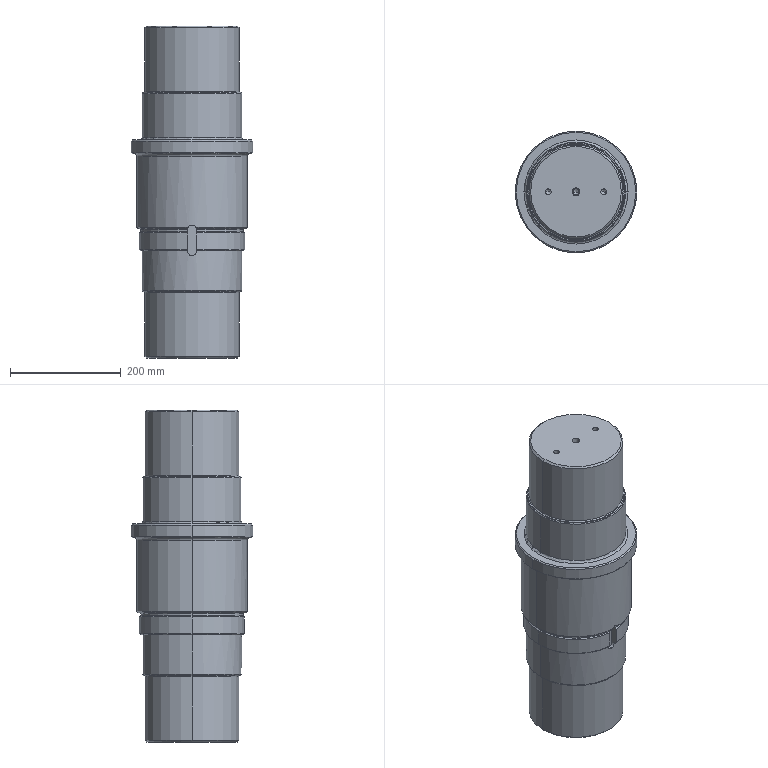Part | SolidWorks | features ICE 9, Chamfer 4, HoleWzd 3, Fillet 2, Extrusion 1, MirrorPattern 1 | 1 solid | 85 faces | box 220 x 220 x 600 mm | volume 15781645 mm3 | cylinder 31 | cone 31 | plane 12 | torus 11 | commonest cylinder face diameters 10.2 x4 170 x4 180 x4 16 x3 186 x3 190 x3